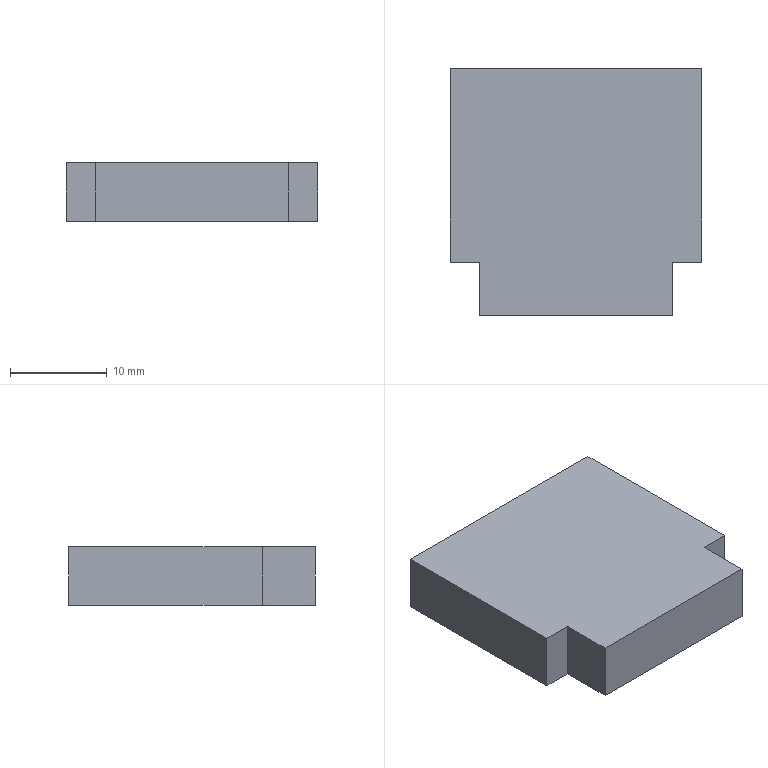Part | SolidWorks | features FlatPattern 1, SMBaseFlange 1, SheetMetal 1 | 1 solid | 10 faces | box 26 x 25.5 x 6 mm | volume 3780 mm3 | plane 10
STEP:
#1=CARTESIAN_POINT('',(15.677,0.,0.));
#2=VERTEX_POINT('',#1);
#3=CARTESIAN_POINT('',(15.677,-5.5,0.));
#4=VERTEX_POINT('',#3);
#5=CARTESIAN_POINT('',(15.677,0.,0.));
#6=DIRECTION('',(0.,-1.,0.));
#7=VECTOR('',#6,1000.);
#8=LINE('',#5,#7);
#9=EDGE_CURVE('',#2,#4,#8,.T.);
#10=ORIENTED_EDGE('',*,*,#9,.T.);
#11=CARTESIAN_POINT('',(15.677,-5.5,6.));
#12=VERTEX_POINT('',#11);
#13=CARTESIAN_POINT('',(15.677,-5.5,6.));
#14=DIRECTION('',(0.,0.,-1.));
#15=VECTOR('',#14,1000.);
#16=LINE('',#13,#15);
#17=EDGE_CURVE('',#12,#4,#16,.T.);
#18=ORIENTED_EDGE('',*,*,#17,.F.);
#19=CARTESIAN_POINT('',(15.677,0.,6.));
#20=VERTEX_POINT('',#19);
#21=CARTESIAN_POINT('',(15.677,0.,6.));
#22=DIRECTION('',(0.,-1.,0.));
#23=VECTOR('',#22,1000.);
#24=LINE('',#21,#23);
#25=EDGE_CURVE('',#20,#12,#24,.T.);
#26=ORIENTED_EDGE('',*,*,#25,.F.);
#27=CARTESIAN_POINT('',(15.677,0.,6.));
#28=DIRECTION('',(0.,0.,-1.));
#29=VECTOR('',#28,1000.);
#30=LINE('',#27,#29);
#31=EDGE_CURVE('',#20,#2,#30,.T.);
#32=ORIENTED_EDGE('',*,*,#31,.T.);
#33=EDGE_LOOP('',(#10,#18,#26,#32));
#34=FACE_OUTER_BOUND('',#33,.T.);
#35=CARTESIAN_POINT('',(15.677,0.,6.));
#36=DIRECTION('',(1.,0.,0.));
#37=DIRECTION('',(0.,1.,0.));
#38=AXIS2_PLACEMENT_3D('',#35,#36,#37);
#39=PLANE('',#38);
#40=ADVANCED_FACE('',(#34),#39,.F.);
#41=CARTESIAN_POINT('',(35.677,-5.5,0.));
#42=VERTEX_POINT('',#41);
#43=CARTESIAN_POINT('',(15.677,-5.5,0.));
#44=DIRECTION('',(1.,0.,0.));
#45=VECTOR('',#44,1000.);
#46=LINE('',#43,#45);
#47=EDGE_CURVE('',#4,#42,#46,.T.);
#48=ORIENTED_EDGE('',*,*,#47,.T.);
#49=CARTESIAN_POINT('',(35.677,-5.5,6.));
#50=VERTEX_POINT('',#49);
#51=CARTESIAN_POINT('',(35.677,-5.5,6.));
#52=DIRECTION('',(0.,0.,-1.));
#53=VECTOR('',#52,1000.);
#54=LINE('',#51,#53);
#55=EDGE_CURVE('',#50,#42,#54,.T.);
#56=ORIENTED_EDGE('',*,*,#55,.F.);
#57=CARTESIAN_POINT('',(15.677,-5.5,6.));
#58=DIRECTION('',(1.,0.,0.));
#59=VECTOR('',#58,1000.);
#60=LINE('',#57,#59);
#61=EDGE_CURVE('',#12,#50,#60,.T.);
#62=ORIENTED_EDGE('',*,*,#61,.F.);
#63=ORIENTED_EDGE('',*,*,#17,.T.);
#64=EDGE_LOOP('',(#48,#56,#62,#63));
#65=FACE_OUTER_BOUND('',#64,.T.);
#66=CARTESIAN_POINT('',(15.677,-5.5,6.));
#67=DIRECTION('',(0.,1.,0.));
#68=DIRECTION('',(0.,0.,1.));
#69=AXIS2_PLACEMENT_3D('',#66,#67,#68);
#70=PLANE('',#69);
#71=ADVANCED_FACE('',(#65),#70,.F.);
#72=CARTESIAN_POINT('',(35.677,0.,0.));
#73=VERTEX_POINT('',#72);
#74=CARTESIAN_POINT('',(35.677,-5.5,0.));
#75=DIRECTION('',(0.,1.,0.));
#76=VECTOR('',#75,1000.);
#77=LINE('',#74,#76);
#78=EDGE_CURVE('',#42,#73,#77,.T.);
#79=ORIENTED_EDGE('',*,*,#78,.T.);
#80=CARTESIAN_POINT('',(35.677,0.,6.));
#81=VERTEX_POINT('',#80);
#82=CARTESIAN_POINT('',(35.677,0.,6.));
#83=DIRECTION('',(0.,0.,-1.));
#84=VECTOR('',#83,1000.);
#85=LINE('',#82,#84);
#86=EDGE_CURVE('',#81,#73,#85,.T.);
#87=ORIENTED_EDGE('',*,*,#86,.F.);
#88=CARTESIAN_POINT('',(35.677,-5.5,6.));
#89=DIRECTION('',(0.,1.,0.));
#90=VECTOR('',#89,1000.);
#91=LINE('',#88,#90);
#92=EDGE_CURVE('',#50,#81,#91,.T.);
#93=ORIENTED_EDGE('',*,*,#92,.F.);
#94=ORIENTED_EDGE('',*,*,#55,.T.);
#95=EDGE_LOOP('',(#79,#87,#93,#94));
#96=FACE_OUTER_BOUND('',#95,.T.);
#97=CARTESIAN_POINT('',(35.677,-5.5,6.));
#98=DIRECTION('',(-1.,0.,0.));
#99=DIRECTION('',(0.,0.,1.));
#100=AXIS2_PLACEMENT_3D('',#97,#98,#99);
#101=PLANE('',#100);
#102=ADVANCED_FACE('',(#96),#101,.F.);
#103=CARTESIAN_POINT('',(38.677,0.,0.));
#104=VERTEX_POINT('',#103);
#105=CARTESIAN_POINT('',(35.677,0.,0.));
#106=DIRECTION('',(1.,0.,0.));
#107=VECTOR('',#106,1000.);
#108=LINE('',#105,#107);
#109=EDGE_CURVE('',#73,#104,#108,.T.);
#110=ORIENTED_EDGE('',*,*,#109,.T.);
#111=CARTESIAN_POINT('',(38.677,0.,6.));
#112=VERTEX_POINT('',#111);
#113=CARTESIAN_POINT('',(38.677,0.,6.));
#114=DIRECTION('',(0.,0.,-1.));
#115=VECTOR('',#114,1000.);
#116=LINE('',#113,#115);
#117=EDGE_CURVE('',#112,#104,#116,.T.);
#118=ORIENTED_EDGE('',*,*,#117,.F.);
#119=CARTESIAN_POINT('',(35.677,0.,6.));
#120=DIRECTION('',(1.,0.,0.));
#121=VECTOR('',#120,1000.);
#122=LINE('',#119,#121);
#123=EDGE_CURVE('',#81,#112,#122,.T.);
#124=ORIENTED_EDGE('',*,*,#123,.F.);
#125=ORIENTED_EDGE('',*,*,#86,.T.);
#126=EDGE_LOOP('',(#110,#118,#124,#125));
#127=FACE_OUTER_BOUND('',#126,.T.);
#128=CARTESIAN_POINT('',(35.677,0.,6.));
#129=DIRECTION('',(0.,1.,0.));
#130=DIRECTION('',(-1.,0.,0.));
#131=AXIS2_PLACEMENT_3D('',#128,#129,#130);
#132=PLANE('',#131);
#133=ADVANCED_FACE('',(#127),#132,.F.);
#134=CARTESIAN_POINT('',(38.677,20.,0.));
#135=VERTEX_POINT('',#134);
#136=CARTESIAN_POINT('',(38.677,0.,0.));
#137=DIRECTION('',(0.,1.,0.));
#138=VECTOR('',#137,1000.);
#139=LINE('',#136,#138);
#140=EDGE_CURVE('',#104,#135,#139,.T.);
#141=ORIENTED_EDGE('',*,*,#140,.T.);
#142=CARTESIAN_POINT('',(38.677,20.,6.));
#143=VERTEX_POINT('',#142);
#144=CARTESIAN_POINT('',(38.677,20.,6.));
#145=DIRECTION('',(0.,0.,-1.));
#146=VECTOR('',#145,1000.);
#147=LINE('',#144,#146);
#148=EDGE_CURVE('',#143,#135,#147,.T.);
#149=ORIENTED_EDGE('',*,*,#148,.F.);
#150=CARTESIAN_POINT('',(38.677,0.,6.));
#151=DIRECTION('',(0.,1.,0.));
#152=VECTOR('',#151,1000.);
#153=LINE('',#150,#152);
#154=EDGE_CURVE('',#112,#143,#153,.T.);
#155=ORIENTED_EDGE('',*,*,#154,.F.);
#156=ORIENTED_EDGE('',*,*,#117,.T.);
#157=EDGE_LOOP('',(#141,#149,#155,#156));
#158=FACE_OUTER_BOUND('',#157,.T.);
#159=CARTESIAN_POINT('',(38.677,0.,6.));
#160=DIRECTION('',(-1.,0.,0.));
#161=DIRECTION('',(0.,0.,1.));
#162=AXIS2_PLACEMENT_3D('',#159,#160,#161);
#163=PLANE('',#162);
#164=ADVANCED_FACE('',(#158),#163,.F.);
#165=CARTESIAN_POINT('',(12.677,20.,0.));
#166=VERTEX_POINT('',#165);
#167=CARTESIAN_POINT('',(38.677,20.,0.));
#168=DIRECTION('',(-1.,0.,0.));
#169=VECTOR('',#168,1000.);
#170=LINE('',#167,#169);
#171=EDGE_CURVE('',#135,#166,#170,.T.);
#172=ORIENTED_EDGE('',*,*,#171,.T.);
#173=CARTESIAN_POINT('',(12.677,20.,6.));
#174=VERTEX_POINT('',#173);
#175=CARTESIAN_POINT('',(12.677,20.,6.));
#176=DIRECTION('',(0.,0.,-1.));
#177=VECTOR('',#176,1000.);
#178=LINE('',#175,#177);
#179=EDGE_CURVE('',#174,#166,#178,.T.);
#180=ORIENTED_EDGE('',*,*,#179,.F.);
#181=CARTESIAN_POINT('',(38.677,20.,6.));
#182=DIRECTION('',(-1.,0.,0.));
#183=VECTOR('',#182,1000.);
#184=LINE('',#181,#183);
#185=EDGE_CURVE('',#143,#174,#184,.T.);
#186=ORIENTED_EDGE('',*,*,#185,.F.);
#187=ORIENTED_EDGE('',*,*,#148,.T.);
#188=EDGE_LOOP('',(#172,#180,#186,#187));
#189=FACE_OUTER_BOUND('',#188,.T.);
#190=CARTESIAN_POINT('',(38.677,20.,6.));
#191=DIRECTION('',(0.,-1.,0.));
#192=DIRECTION('',(1.,0.,0.));
#193=AXIS2_PLACEMENT_3D('',#190,#191,#192);
#194=PLANE('',#193);
#195=ADVANCED_FACE('',(#189),#194,.F.);
#196=CARTESIAN_POINT('',(12.677,0.,0.));
#197=VERTEX_POINT('',#196);
#198=CARTESIAN_POINT('',(12.677,20.,0.));
#199=DIRECTION('',(0.,-1.,0.));
#200=VECTOR('',#199,1000.);
#201=LINE('',#198,#200);
#202=EDGE_CURVE('',#166,#197,#201,.T.);
#203=ORIENTED_EDGE('',*,*,#202,.T.);
#204=CARTESIAN_POINT('',(12.677,0.,6.));
#205=VERTEX_POINT('',#204);
#206=CARTESIAN_POINT('',(12.677,0.,6.));
#207=DIRECTION('',(0.,0.,-1.));
#208=VECTOR('',#207,1000.);
#209=LINE('',#206,#208);
#210=EDGE_CURVE('',#205,#197,#209,.T.);
#211=ORIENTED_EDGE('',*,*,#210,.F.);
#212=CARTESIAN_POINT('',(12.677,20.,6.));
#213=DIRECTION('',(0.,-1.,0.));
#214=VECTOR('',#213,1000.);
#215=LINE('',#212,#214);
#216=EDGE_CURVE('',#174,#205,#215,.T.);
#217=ORIENTED_EDGE('',*,*,#216,.F.);
#218=ORIENTED_EDGE('',*,*,#179,.T.);
#219=EDGE_LOOP('',(#203,#211,#217,#218));
#220=FACE_OUTER_BOUND('',#219,.T.);
#221=CARTESIAN_POINT('',(12.677,20.,6.));
#222=DIRECTION('',(1.,0.,0.));
#223=DIRECTION('',(0.,0.,-1.));
#224=AXIS2_PLACEMENT_3D('',#221,#222,#223);
#225=PLANE('',#224);
#226=ADVANCED_FACE('',(#220),#225,.F.);
#227=CARTESIAN_POINT('',(15.677,0.,0.));
#228=DIRECTION('',(1.,0.,0.));
#229=VECTOR('',#228,1000.);
#230=LINE('',#227,#229);
#231=EDGE_CURVE('',#197,#2,#230,.T.);
#232=ORIENTED_EDGE('',*,*,#231,.T.);
#233=ORIENTED_EDGE('',*,*,#31,.F.);
#234=CARTESIAN_POINT('',(15.677,0.,6.));
#235=DIRECTION('',(1.,0.,0.));
#236=VECTOR('',#235,1000.);
#237=LINE('',#234,#236);
#238=EDGE_CURVE('',#205,#20,#237,.T.);
#239=ORIENTED_EDGE('',*,*,#238,.F.);
#240=ORIENTED_EDGE('',*,*,#210,.T.);
#241=EDGE_LOOP('',(#232,#233,#239,#240));
#242=FACE_OUTER_BOUND('',#241,.T.);
#243=CARTESIAN_POINT('',(15.677,0.,6.));
#244=DIRECTION('',(0.,1.,0.));
#245=DIRECTION('',(-1.,0.,0.));
#246=AXIS2_PLACEMENT_3D('',#243,#244,#245);
#247=PLANE('',#246);
#248=ADVANCED_FACE('',(#242),#247,.F.);
#249=ORIENTED_EDGE('',*,*,#25,.T.);
#250=ORIENTED_EDGE('',*,*,#61,.T.);
#251=ORIENTED_EDGE('',*,*,#92,.T.);
#252=ORIENTED_EDGE('',*,*,#123,.T.);
#253=ORIENTED_EDGE('',*,*,#154,.T.);
#254=ORIENTED_EDGE('',*,*,#185,.T.);
#255=ORIENTED_EDGE('',*,*,#216,.T.);
#256=ORIENTED_EDGE('',*,*,#238,.T.);
#257=EDGE_LOOP('',(#249,#250,#251,#252,#253,#254,#255,#256));
#258=FACE_OUTER_BOUND('',#257,.T.);
#259=CARTESIAN_POINT('',(0.,0.,6.));
#260=DIRECTION('',(0.,0.,1.));
#261=DIRECTION('',(1.,0.,0.));
#262=AXIS2_PLACEMENT_3D('',#259,#260,#261);
#263=PLANE('',#262);
#264=ADVANCED_FACE('',(#258),#263,.T.);
#265=ORIENTED_EDGE('',*,*,#9,.F.);
#266=ORIENTED_EDGE('',*,*,#231,.F.);
#267=ORIENTED_EDGE('',*,*,#202,.F.);
#268=ORIENTED_EDGE('',*,*,#171,.F.);
#269=ORIENTED_EDGE('',*,*,#140,.F.);
#270=ORIENTED_EDGE('',*,*,#109,.F.);
#271=ORIENTED_EDGE('',*,*,#78,.F.);
#272=ORIENTED_EDGE('',*,*,#47,.F.);
#273=EDGE_LOOP('',(#265,#266,#267,#268,#269,#270,#271,#272));
#274=FACE_OUTER_BOUND('',#273,.T.);
#275=CARTESIAN_POINT('',(0.,0.,0.));
#276=DIRECTION('',(0.,0.,1.));
#277=DIRECTION('',(1.,0.,0.));
#278=AXIS2_PLACEMENT_3D('',#275,#276,#277);
#279=PLANE('',#278);
#280=ADVANCED_FACE('',(#274),#279,.F.);
#281=CLOSED_SHELL('',(#40,#71,#102,#133,#164,#195,#226,#248,#264,#280));
#282=MANIFOLD_SOLID_BREP('',#281);
#283=CARTESIAN_POINT('',(0.,0.,0.));
#284=DIRECTION('',(0.,0.,1.));
#285=DIRECTION('',(1.,0.,0.));
#286=AXIS2_PLACEMENT_3D('',#283,#284,#285);
#287=(LENGTH_UNIT()NAMED_UNIT(*)SI_UNIT(.MILLI.,.METRE.));
#288=UNCERTAINTY_MEASURE_WITH_UNIT(LENGTH_MEASURE(0.00001),#287,'','');
#289=(NAMED_UNIT(*)PLANE_ANGLE_UNIT()SI_UNIT($,.RADIAN.));
#290=(NAMED_UNIT(*)SI_UNIT($,.STERADIAN.)SOLID_ANGLE_UNIT());
#291=(GEOMETRIC_REPRESENTATION_CONTEXT(3)GLOBAL_UNCERTAINTY_ASSIGNED_CONTEXT((#288))GLOBAL_UNIT_ASSIGNED_CONTEXT((#287,#289,#290))REPRESENTATION_CONTEXT('',''));
#292=ADVANCED_BREP_SHAPE_REPRESENTATION('',(#282,#286),#291);